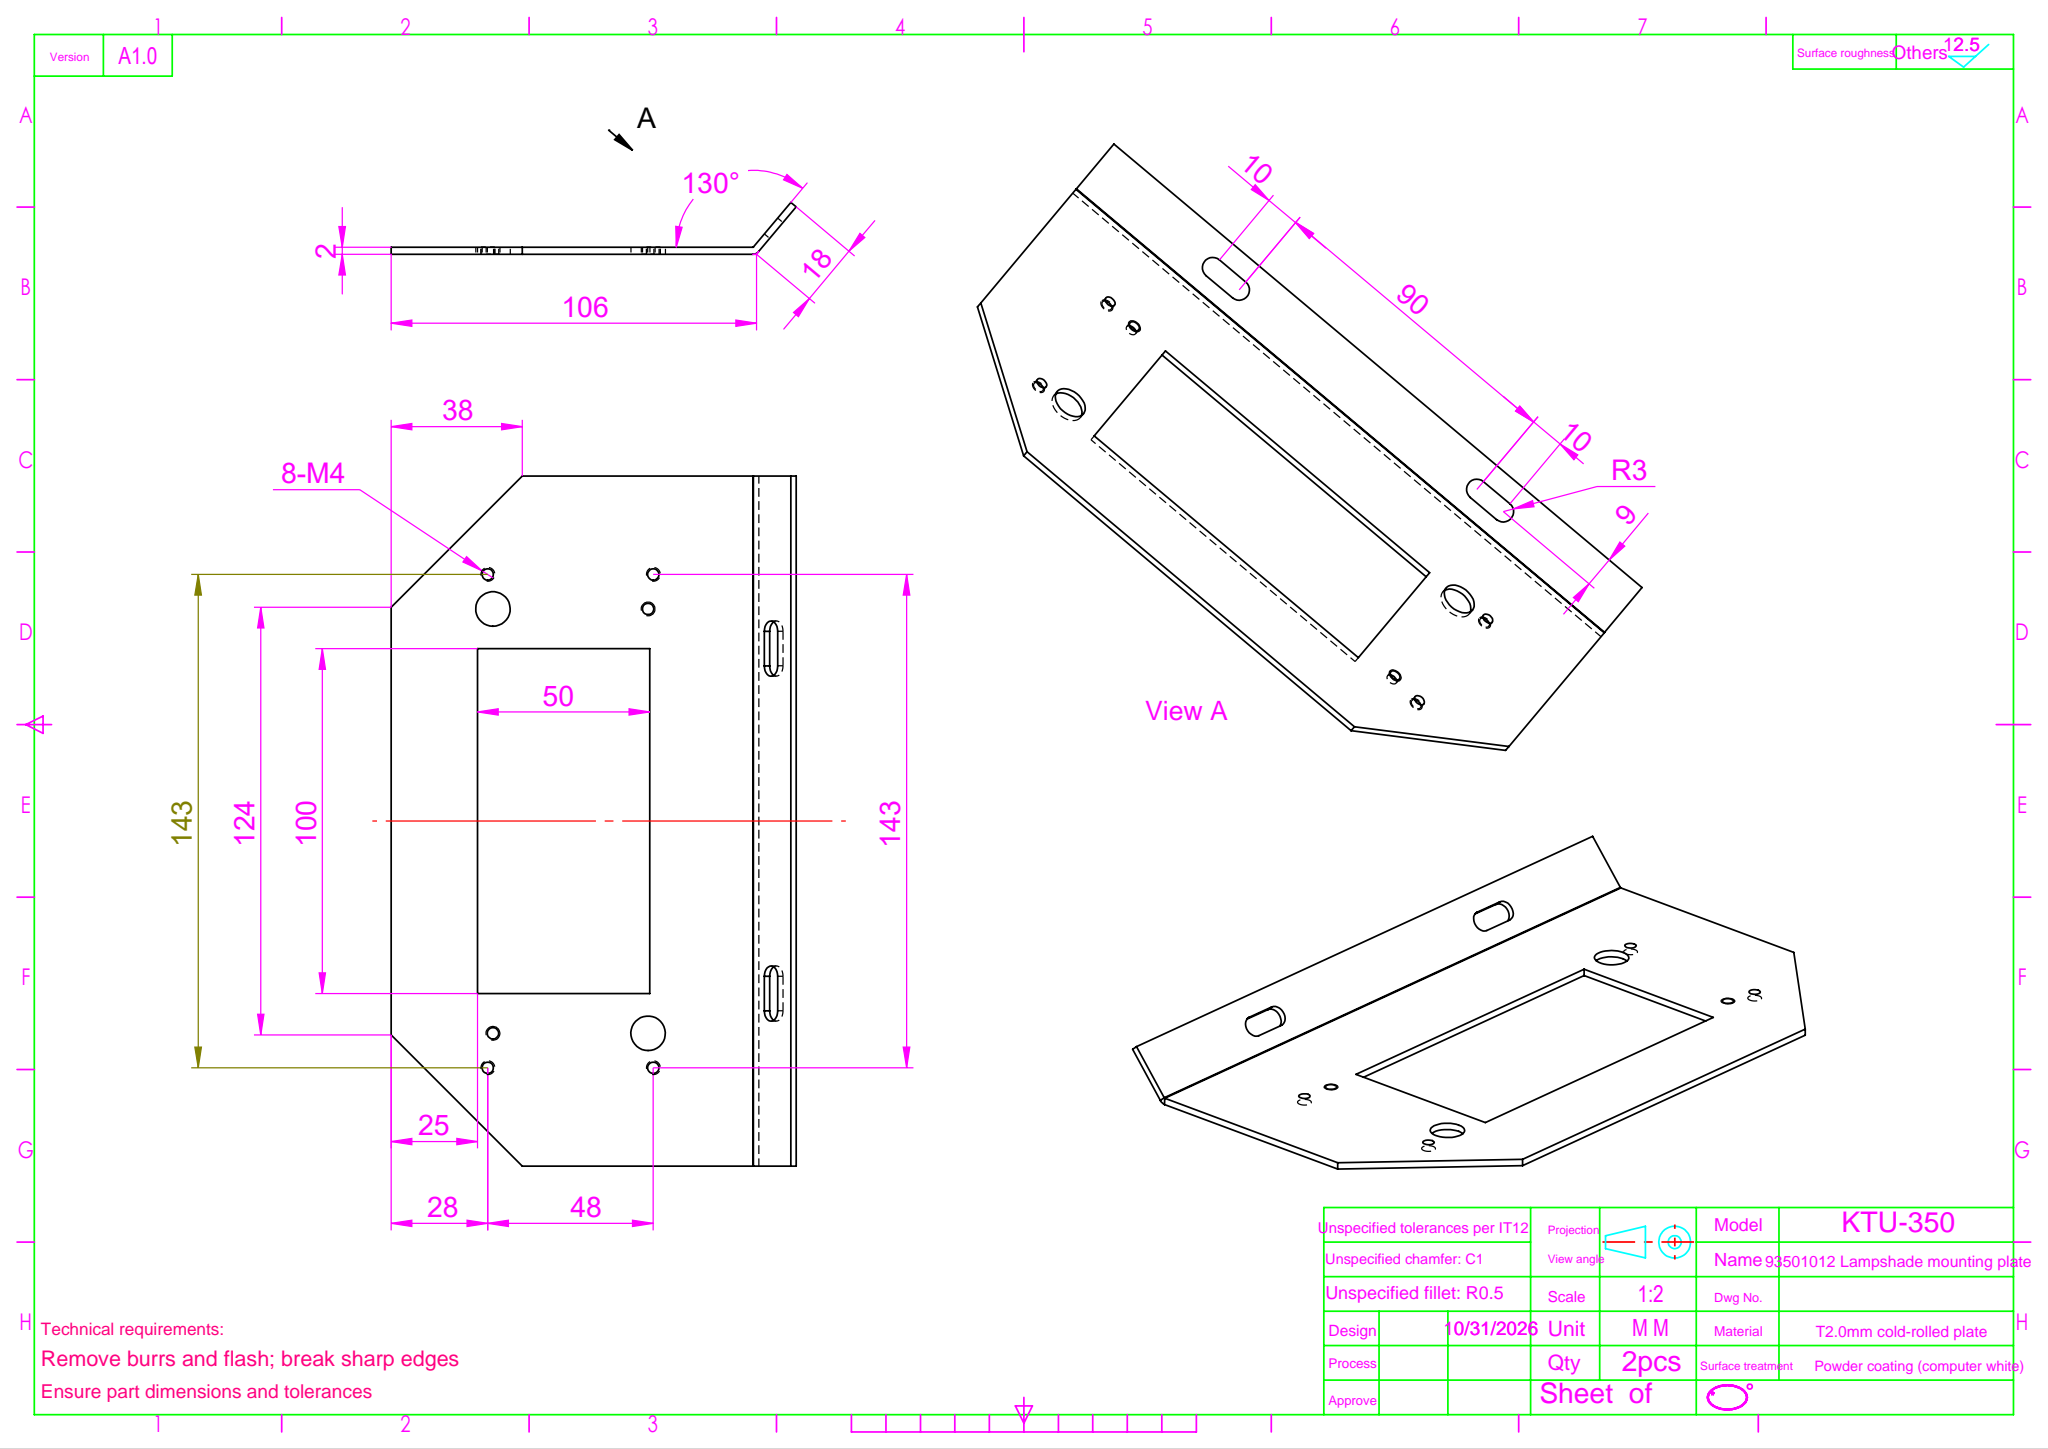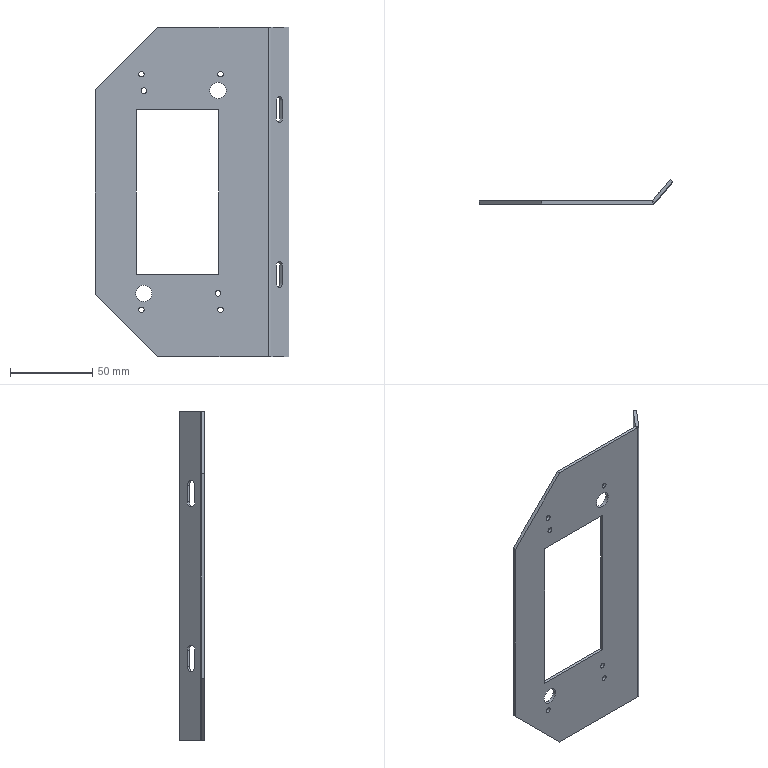Part | SolidWorks | features ICE 3, HoleWzd 2, Chamfer 1, FlatPattern 1, SMBaseFlange 1, SheetMetal 1 | 1 solid | 44 faces | box 117.459 x 15.023 x 200 mm | volume 35486 mm3 | cylinder 22 | plane 22 | commonest cylinder face diameters 3.3 x12 6 x4 10 x4 0.4 x1 4.4 x1